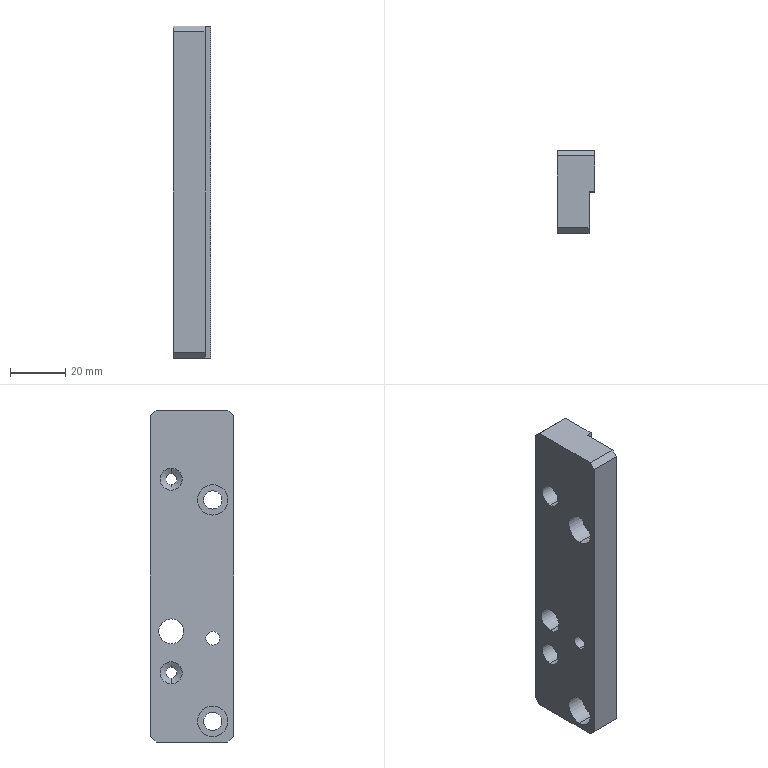Part | SolidWorks | features HoleWzd 5, Chamfer 1, Cut 1, Extrusion 1 | 1 solid | 38 faces | box 13.4 x 30 x 120 mm | volume 40915 mm3 | cylinder 20 | plane 14 | cone 4 | commonest cylinder face diameters 4 x4 6.6 x4 8 x4 11 x4 5 x2 9 x2
STEP:
#1=CARTESIAN_POINT('',(11.4,-7.5,-25.));
#2=VERTEX_POINT('',#1);
#3=CARTESIAN_POINT('',(11.4,-7.5,-20.));
#4=VERTEX_POINT('',#3);
#5=CARTESIAN_POINT('',(11.4,-7.5,-22.5));
#6=DIRECTION('',(-1.,0.,0.));
#7=DIRECTION('',(0.,0.,1.));
#8=AXIS2_PLACEMENT_3D('',#5,#6,#7);
#9=CIRCLE('',#8,2.5);
#10=EDGE_CURVE('',#2,#4,#9,.T.);
#11=ORIENTED_EDGE('',*,*,#10,.F.);
#12=CARTESIAN_POINT('',(0.,-7.5,-25.));
#13=VERTEX_POINT('',#12);
#14=CARTESIAN_POINT('',(0.,-7.5,-25.));
#15=DIRECTION('',(-1.,0.,0.));
#16=VECTOR('',#15,1000.);
#17=LINE('',#14,#16);
#18=EDGE_CURVE('',#2,#13,#17,.T.);
#19=ORIENTED_EDGE('',*,*,#18,.T.);
#20=CARTESIAN_POINT('',(0.,-7.5,-20.));
#21=VERTEX_POINT('',#20);
#22=CARTESIAN_POINT('',(0.,-7.5,-22.5));
#23=DIRECTION('',(-1.,0.,0.));
#24=DIRECTION('',(0.,0.,1.));
#25=AXIS2_PLACEMENT_3D('',#22,#23,#24);
#26=CIRCLE('',#25,2.5);
#27=EDGE_CURVE('',#13,#21,#26,.T.);
#28=ORIENTED_EDGE('',*,*,#27,.T.);
#29=CARTESIAN_POINT('',(0.,-7.5,-20.));
#30=DIRECTION('',(-1.,0.,0.));
#31=VECTOR('',#30,1000.);
#32=LINE('',#29,#31);
#33=EDGE_CURVE('',#4,#21,#32,.T.);
#34=ORIENTED_EDGE('',*,*,#33,.F.);
#35=EDGE_LOOP('',(#11,#19,#28,#34));
#36=FACE_OUTER_BOUND('',#35,.T.);
#37=CARTESIAN_POINT('',(0.,-7.5,-22.5));
#38=DIRECTION('',(-1.,0.,0.));
#39=DIRECTION('',(0.,0.,1.));
#40=AXIS2_PLACEMENT_3D('',#37,#38,#39);
#41=CYLINDRICAL_SURFACE('',#40,2.5);
#42=ADVANCED_FACE('',(#36),#41,.F.);
#43=CARTESIAN_POINT('',(6.8,-7.5,-58.));
#44=VERTEX_POINT('',#43);
#45=CARTESIAN_POINT('',(6.8,-7.5,-47.));
#46=VERTEX_POINT('',#45);
#47=CARTESIAN_POINT('',(6.8,-7.5,-52.5));
#48=DIRECTION('',(-1.,0.,0.));
#49=DIRECTION('',(0.,0.,1.));
#50=AXIS2_PLACEMENT_3D('',#47,#48,#49);
#51=CIRCLE('',#50,5.5);
#52=EDGE_CURVE('',#44,#46,#51,.T.);
#53=ORIENTED_EDGE('',*,*,#52,.F.);
#54=CARTESIAN_POINT('',(0.,-7.5,-58.));
#55=VERTEX_POINT('',#54);
#56=CARTESIAN_POINT('',(0.,-7.5,-58.));
#57=DIRECTION('',(-1.,0.,0.));
#58=VECTOR('',#57,1000.);
#59=LINE('',#56,#58);
#60=EDGE_CURVE('',#44,#55,#59,.T.);
#61=ORIENTED_EDGE('',*,*,#60,.T.);
#62=CARTESIAN_POINT('',(0.,-7.5,-47.));
#63=VERTEX_POINT('',#62);
#64=CARTESIAN_POINT('',(0.,-7.5,-52.5));
#65=DIRECTION('',(-1.,0.,0.));
#66=DIRECTION('',(0.,0.,1.));
#67=AXIS2_PLACEMENT_3D('',#64,#65,#66);
#68=CIRCLE('',#67,5.5);
#69=EDGE_CURVE('',#55,#63,#68,.T.);
#70=ORIENTED_EDGE('',*,*,#69,.T.);
#71=CARTESIAN_POINT('',(0.,-7.5,-47.));
#72=DIRECTION('',(-1.,0.,0.));
#73=VECTOR('',#72,1000.);
#74=LINE('',#71,#73);
#75=EDGE_CURVE('',#46,#63,#74,.T.);
#76=ORIENTED_EDGE('',*,*,#75,.F.);
#77=EDGE_LOOP('',(#53,#61,#70,#76));
#78=FACE_OUTER_BOUND('',#77,.T.);
#79=CARTESIAN_POINT('',(0.,-7.5,-52.5));
#80=DIRECTION('',(-1.,0.,0.));
#81=DIRECTION('',(0.,0.,1.));
#82=AXIS2_PLACEMENT_3D('',#79,#80,#81);
#83=CYLINDRICAL_SURFACE('',#82,5.5);
#84=ADVANCED_FACE('',(#78),#83,.F.);
#85=CARTESIAN_POINT('',(11.4,-7.5,-55.8));
#86=VERTEX_POINT('',#85);
#87=CARTESIAN_POINT('',(11.4,-7.5,-49.2));
#88=VERTEX_POINT('',#87);
#89=CARTESIAN_POINT('',(11.4,-7.5,-52.5));
#90=DIRECTION('',(-1.,0.,0.));
#91=DIRECTION('',(0.,0.,1.));
#92=AXIS2_PLACEMENT_3D('',#89,#90,#91);
#93=CIRCLE('',#92,3.3);
#94=EDGE_CURVE('',#86,#88,#93,.T.);
#95=ORIENTED_EDGE('',*,*,#94,.F.);
#96=CARTESIAN_POINT('',(6.8,-7.5,-55.8));
#97=VERTEX_POINT('',#96);
#98=CARTESIAN_POINT('',(0.,-7.5,-55.8));
#99=DIRECTION('',(-1.,0.,0.));
#100=VECTOR('',#99,1000.);
#101=LINE('',#98,#100);
#102=EDGE_CURVE('',#86,#97,#101,.T.);
#103=ORIENTED_EDGE('',*,*,#102,.T.);
#104=CARTESIAN_POINT('',(6.8,-7.5,-49.2));
#105=VERTEX_POINT('',#104);
#106=CARTESIAN_POINT('',(6.8,-7.5,-52.5));
#107=DIRECTION('',(-1.,0.,0.));
#108=DIRECTION('',(0.,0.,1.));
#109=AXIS2_PLACEMENT_3D('',#106,#107,#108);
#110=CIRCLE('',#109,3.3);
#111=EDGE_CURVE('',#97,#105,#110,.T.);
#112=ORIENTED_EDGE('',*,*,#111,.T.);
#113=CARTESIAN_POINT('',(0.,-7.5,-49.2));
#114=DIRECTION('',(-1.,0.,0.));
#115=VECTOR('',#114,1000.);
#116=LINE('',#113,#115);
#117=EDGE_CURVE('',#88,#105,#116,.T.);
#118=ORIENTED_EDGE('',*,*,#117,.F.);
#119=EDGE_LOOP('',(#95,#103,#112,#118));
#120=FACE_OUTER_BOUND('',#119,.T.);
#121=CARTESIAN_POINT('',(0.,-7.5,-52.5));
#122=DIRECTION('',(-1.,0.,0.));
#123=DIRECTION('',(0.,0.,1.));
#124=AXIS2_PLACEMENT_3D('',#121,#122,#123);
#125=CYLINDRICAL_SURFACE('',#124,3.3);
#126=ADVANCED_FACE('',(#120),#125,.F.);
#127=CARTESIAN_POINT('',(6.8,-7.5,22.));
#128=VERTEX_POINT('',#127);
#129=CARTESIAN_POINT('',(6.8,-7.5,33.));
#130=VERTEX_POINT('',#129);
#131=CARTESIAN_POINT('',(6.8,-7.5,27.5));
#132=DIRECTION('',(-1.,0.,0.));
#133=DIRECTION('',(0.,0.,1.));
#134=AXIS2_PLACEMENT_3D('',#131,#132,#133);
#135=CIRCLE('',#134,5.5);
#136=EDGE_CURVE('',#128,#130,#135,.T.);
#137=ORIENTED_EDGE('',*,*,#136,.F.);
#138=CARTESIAN_POINT('',(0.,-7.5,22.));
#139=VERTEX_POINT('',#138);
#140=CARTESIAN_POINT('',(0.,-7.5,22.));
#141=DIRECTION('',(-1.,0.,0.));
#142=VECTOR('',#141,1000.);
#143=LINE('',#140,#142);
#144=EDGE_CURVE('',#128,#139,#143,.T.);
#145=ORIENTED_EDGE('',*,*,#144,.T.);
#146=CARTESIAN_POINT('',(0.,-7.5,33.));
#147=VERTEX_POINT('',#146);
#148=CARTESIAN_POINT('',(0.,-7.5,27.5));
#149=DIRECTION('',(-1.,0.,0.));
#150=DIRECTION('',(0.,0.,1.));
#151=AXIS2_PLACEMENT_3D('',#148,#149,#150);
#152=CIRCLE('',#151,5.5);
#153=EDGE_CURVE('',#139,#147,#152,.T.);
#154=ORIENTED_EDGE('',*,*,#153,.T.);
#155=CARTESIAN_POINT('',(0.,-7.5,33.));
#156=DIRECTION('',(-1.,0.,0.));
#157=VECTOR('',#156,1000.);
#158=LINE('',#155,#157);
#159=EDGE_CURVE('',#130,#147,#158,.T.);
#160=ORIENTED_EDGE('',*,*,#159,.F.);
#161=EDGE_LOOP('',(#137,#145,#154,#160));
#162=FACE_OUTER_BOUND('',#161,.T.);
#163=CARTESIAN_POINT('',(0.,-7.5,27.5));
#164=DIRECTION('',(-1.,0.,0.));
#165=DIRECTION('',(0.,0.,1.));
#166=AXIS2_PLACEMENT_3D('',#163,#164,#165);
#167=CYLINDRICAL_SURFACE('',#166,5.5);
#168=ADVANCED_FACE('',(#162),#167,.F.);
#169=CARTESIAN_POINT('',(11.4,-7.5,24.2));
#170=VERTEX_POINT('',#169);
#171=CARTESIAN_POINT('',(11.4,-7.5,30.8));
#172=VERTEX_POINT('',#171);
#173=CARTESIAN_POINT('',(11.4,-7.5,27.5));
#174=DIRECTION('',(-1.,0.,0.));
#175=DIRECTION('',(0.,0.,1.));
#176=AXIS2_PLACEMENT_3D('',#173,#174,#175);
#177=CIRCLE('',#176,3.3);
#178=EDGE_CURVE('',#170,#172,#177,.T.);
#179=ORIENTED_EDGE('',*,*,#178,.F.);
#180=CARTESIAN_POINT('',(6.8,-7.5,24.2));
#181=VERTEX_POINT('',#180);
#182=CARTESIAN_POINT('',(0.,-7.5,24.2));
#183=DIRECTION('',(-1.,0.,0.));
#184=VECTOR('',#183,1000.);
#185=LINE('',#182,#184);
#186=EDGE_CURVE('',#170,#181,#185,.T.);
#187=ORIENTED_EDGE('',*,*,#186,.T.);
#188=CARTESIAN_POINT('',(6.8,-7.5,30.8));
#189=VERTEX_POINT('',#188);
#190=CARTESIAN_POINT('',(6.8,-7.5,27.5));
#191=DIRECTION('',(-1.,0.,0.));
#192=DIRECTION('',(0.,0.,1.));
#193=AXIS2_PLACEMENT_3D('',#190,#191,#192);
#194=CIRCLE('',#193,3.3);
#195=EDGE_CURVE('',#181,#189,#194,.T.);
#196=ORIENTED_EDGE('',*,*,#195,.T.);
#197=CARTESIAN_POINT('',(0.,-7.5,30.8));
#198=DIRECTION('',(-1.,0.,0.));
#199=VECTOR('',#198,1000.);
#200=LINE('',#197,#199);
#201=EDGE_CURVE('',#172,#189,#200,.T.);
#202=ORIENTED_EDGE('',*,*,#201,.F.);
#203=EDGE_LOOP('',(#179,#187,#196,#202));
#204=FACE_OUTER_BOUND('',#203,.T.);
#205=CARTESIAN_POINT('',(0.,-7.5,27.5));
#206=DIRECTION('',(-1.,0.,0.));
#207=DIRECTION('',(0.,0.,1.));
#208=AXIS2_PLACEMENT_3D('',#205,#206,#207);
#209=CYLINDRICAL_SURFACE('',#208,3.3);
#210=ADVANCED_FACE('',(#204),#209,.F.);
#211=CARTESIAN_POINT('',(0.,7.5,-15.5));
#212=VERTEX_POINT('',#211);
#213=CARTESIAN_POINT('',(0.,7.5,-24.5));
#214=VERTEX_POINT('',#213);
#215=CARTESIAN_POINT('',(0.,7.5,-20.));
#216=DIRECTION('',(1.,0.,0.));
#217=DIRECTION('',(0.,0.,-1.));
#218=AXIS2_PLACEMENT_3D('',#215,#216,#217);
#219=CIRCLE('',#218,4.5);
#220=EDGE_CURVE('',#212,#214,#219,.T.);
#221=ORIENTED_EDGE('',*,*,#220,.F.);
#222=CARTESIAN_POINT('',(13.4,7.5,-15.5));
#223=VERTEX_POINT('',#222);
#224=CARTESIAN_POINT('',(13.4,7.5,-15.5));
#225=DIRECTION('',(1.,0.,0.));
#226=VECTOR('',#225,1000.);
#227=LINE('',#224,#226);
#228=EDGE_CURVE('',#212,#223,#227,.T.);
#229=ORIENTED_EDGE('',*,*,#228,.T.);
#230=CARTESIAN_POINT('',(13.4,7.5,-24.5));
#231=VERTEX_POINT('',#230);
#232=CARTESIAN_POINT('',(13.4,7.5,-20.));
#233=DIRECTION('',(1.,0.,0.));
#234=DIRECTION('',(0.,0.,-1.));
#235=AXIS2_PLACEMENT_3D('',#232,#233,#234);
#236=CIRCLE('',#235,4.5);
#237=EDGE_CURVE('',#223,#231,#236,.T.);
#238=ORIENTED_EDGE('',*,*,#237,.T.);
#239=CARTESIAN_POINT('',(13.4,7.5,-24.5));
#240=DIRECTION('',(1.,0.,0.));
#241=VECTOR('',#240,1000.);
#242=LINE('',#239,#241);
#243=EDGE_CURVE('',#214,#231,#242,.T.);
#244=ORIENTED_EDGE('',*,*,#243,.F.);
#245=EDGE_LOOP('',(#221,#229,#238,#244));
#246=FACE_OUTER_BOUND('',#245,.T.);
#247=CARTESIAN_POINT('',(13.4,7.5,-20.));
#248=DIRECTION('',(1.,0.,0.));
#249=DIRECTION('',(0.,0.,-1.));
#250=AXIS2_PLACEMENT_3D('',#247,#248,#249);
#251=CYLINDRICAL_SURFACE('',#250,4.5);
#252=ADVANCED_FACE('',(#246),#251,.F.);
#253=CARTESIAN_POINT('',(7.5,7.5,31.));
#254=VERTEX_POINT('',#253);
#255=CARTESIAN_POINT('',(7.5,7.5,39.));
#256=VERTEX_POINT('',#255);
#257=CARTESIAN_POINT('',(7.5,7.5,35.));
#258=DIRECTION('',(-1.,0.,0.));
#259=DIRECTION('',(0.,0.,1.));
#260=AXIS2_PLACEMENT_3D('',#257,#258,#259);
#261=CIRCLE('',#260,4.);
#262=EDGE_CURVE('',#254,#256,#261,.T.);
#263=ORIENTED_EDGE('',*,*,#262,.F.);
#264=CARTESIAN_POINT('',(0.,7.5,31.));
#265=VERTEX_POINT('',#264);
#266=CARTESIAN_POINT('',(0.,7.5,31.));
#267=DIRECTION('',(-1.,0.,0.));
#268=VECTOR('',#267,1000.);
#269=LINE('',#266,#268);
#270=EDGE_CURVE('',#254,#265,#269,.T.);
#271=ORIENTED_EDGE('',*,*,#270,.T.);
#272=CARTESIAN_POINT('',(0.,7.5,39.));
#273=VERTEX_POINT('',#272);
#274=CARTESIAN_POINT('',(0.,7.5,35.));
#275=DIRECTION('',(-1.,0.,0.));
#276=DIRECTION('',(0.,0.,1.));
#277=AXIS2_PLACEMENT_3D('',#274,#275,#276);
#278=CIRCLE('',#277,4.);
#279=EDGE_CURVE('',#265,#273,#278,.T.);
#280=ORIENTED_EDGE('',*,*,#279,.T.);
#281=CARTESIAN_POINT('',(0.,7.5,39.));
#282=DIRECTION('',(-1.,0.,0.));
#283=VECTOR('',#282,1000.);
#284=LINE('',#281,#283);
#285=EDGE_CURVE('',#256,#273,#284,.T.);
#286=ORIENTED_EDGE('',*,*,#285,.F.);
#287=EDGE_LOOP('',(#263,#271,#280,#286));
#288=FACE_OUTER_BOUND('',#287,.T.);
#289=CARTESIAN_POINT('',(0.,7.5,35.));
#290=DIRECTION('',(-1.,0.,0.));
#291=DIRECTION('',(0.,0.,1.));
#292=AXIS2_PLACEMENT_3D('',#289,#290,#291);
#293=CYLINDRICAL_SURFACE('',#292,4.);
#294=ADVANCED_FACE('',(#288),#293,.F.);
#295=CARTESIAN_POINT('',(8.702,7.5,33.));
#296=VERTEX_POINT('',#295);
#297=CARTESIAN_POINT('',(8.702,7.5,37.));
#298=VERTEX_POINT('',#297);
#299=CARTESIAN_POINT('',(8.702,7.5,35.));
#300=DIRECTION('',(-1.,0.,0.));
#301=DIRECTION('',(0.,0.,1.));
#302=AXIS2_PLACEMENT_3D('',#299,#300,#301);
#303=CIRCLE('',#302,2.);
#304=EDGE_CURVE('',#296,#298,#303,.T.);
#305=ORIENTED_EDGE('',*,*,#304,.F.);
#306=CARTESIAN_POINT('',(7.5,7.5,31.));
#307=DIRECTION('',(-0.515,0.,-0.8572));
#308=VECTOR('',#307,1000.);
#309=LINE('',#306,#308);
#310=EDGE_CURVE('',#296,#254,#309,.T.);
#311=ORIENTED_EDGE('',*,*,#310,.T.);
#312=ORIENTED_EDGE('',*,*,#262,.T.);
#313=CARTESIAN_POINT('',(7.5,7.5,39.));
#314=DIRECTION('',(-0.515,0.,0.8572));
#315=VECTOR('',#314,1000.);
#316=LINE('',#313,#315);
#317=EDGE_CURVE('',#298,#256,#316,.T.);
#318=ORIENTED_EDGE('',*,*,#317,.F.);
#319=EDGE_LOOP('',(#305,#311,#312,#318));
#320=FACE_OUTER_BOUND('',#319,.T.);
#321=CARTESIAN_POINT('',(7.5,7.5,35.));
#322=DIRECTION('',(-1.,0.,0.));
#323=DIRECTION('',(0.,0.,1.));
#324=AXIS2_PLACEMENT_3D('',#321,#322,#323);
#325=CONICAL_SURFACE('',#324,4.,1.03);
#326=ADVANCED_FACE('',(#320),#325,.F.);
#327=CARTESIAN_POINT('',(13.4,7.5,33.));
#328=VERTEX_POINT('',#327);
#329=CARTESIAN_POINT('',(13.4,7.5,37.));
#330=VERTEX_POINT('',#329);
#331=CARTESIAN_POINT('',(13.4,7.5,35.));
#332=DIRECTION('',(-1.,0.,0.));
#333=DIRECTION('',(0.,0.,1.));
#334=AXIS2_PLACEMENT_3D('',#331,#332,#333);
#335=CIRCLE('',#334,2.);
#336=EDGE_CURVE('',#328,#330,#335,.T.);
#337=ORIENTED_EDGE('',*,*,#336,.F.);
#338=CARTESIAN_POINT('',(0.,7.5,33.));
#339=DIRECTION('',(-1.,0.,0.));
#340=VECTOR('',#339,1000.);
#341=LINE('',#338,#340);
#342=EDGE_CURVE('',#328,#296,#341,.T.);
#343=ORIENTED_EDGE('',*,*,#342,.T.);
#344=ORIENTED_EDGE('',*,*,#304,.T.);
#345=CARTESIAN_POINT('',(0.,7.5,37.));
#346=DIRECTION('',(-1.,0.,0.));
#347=VECTOR('',#346,1000.);
#348=LINE('',#345,#347);
#349=EDGE_CURVE('',#330,#298,#348,.T.);
#350=ORIENTED_EDGE('',*,*,#349,.F.);
#351=EDGE_LOOP('',(#337,#343,#344,#350));
#352=FACE_OUTER_BOUND('',#351,.T.);
#353=CARTESIAN_POINT('',(0.,7.5,35.));
#354=DIRECTION('',(-1.,0.,0.));
#355=DIRECTION('',(0.,0.,1.));
#356=AXIS2_PLACEMENT_3D('',#353,#354,#355);
#357=CYLINDRICAL_SURFACE('',#356,2.);
#358=ADVANCED_FACE('',(#352),#357,.F.);
#359=CARTESIAN_POINT('',(7.5,7.5,-39.));
#360=VERTEX_POINT('',#359);
#361=CARTESIAN_POINT('',(7.5,7.5,-31.));
#362=VERTEX_POINT('',#361);
#363=CARTESIAN_POINT('',(7.5,7.5,-35.));
#364=DIRECTION('',(-1.,0.,0.));
#365=DIRECTION('',(0.,0.,1.));
#366=AXIS2_PLACEMENT_3D('',#363,#364,#365);
#367=CIRCLE('',#366,4.);
#368=EDGE_CURVE('',#360,#362,#367,.T.);
#369=ORIENTED_EDGE('',*,*,#368,.F.);
#370=CARTESIAN_POINT('',(0.,7.5,-39.));
#371=VERTEX_POINT('',#370);
#372=CARTESIAN_POINT('',(0.,7.5,-39.));
#373=DIRECTION('',(-1.,0.,0.));
#374=VECTOR('',#373,1000.);
#375=LINE('',#372,#374);
#376=EDGE_CURVE('',#360,#371,#375,.T.);
#377=ORIENTED_EDGE('',*,*,#376,.T.);
#378=CARTESIAN_POINT('',(0.,7.5,-31.));
#379=VERTEX_POINT('',#378);
#380=CARTESIAN_POINT('',(0.,7.5,-35.));
#381=DIRECTION('',(-1.,0.,0.));
#382=DIRECTION('',(0.,0.,1.));
#383=AXIS2_PLACEMENT_3D('',#380,#381,#382);
#384=CIRCLE('',#383,4.);
#385=EDGE_CURVE('',#371,#379,#384,.T.);
#386=ORIENTED_EDGE('',*,*,#385,.T.);
#387=CARTESIAN_POINT('',(0.,7.5,-31.));
#388=DIRECTION('',(-1.,0.,0.));
#389=VECTOR('',#388,1000.);
#390=LINE('',#387,#389);
#391=EDGE_CURVE('',#362,#379,#390,.T.);
#392=ORIENTED_EDGE('',*,*,#391,.F.);
#393=EDGE_LOOP('',(#369,#377,#386,#392));
#394=FACE_OUTER_BOUND('',#393,.T.);
#395=CARTESIAN_POINT('',(0.,7.5,-35.));
#396=DIRECTION('',(-1.,0.,0.));
#397=DIRECTION('',(0.,0.,1.));
#398=AXIS2_PLACEMENT_3D('',#395,#396,#397);
#399=CYLINDRICAL_SURFACE('',#398,4.);
#400=ADVANCED_FACE('',(#394),#399,.F.);
#401=CARTESIAN_POINT('',(8.702,7.5,-37.));
#402=VERTEX_POINT('',#401);
#403=CARTESIAN_POINT('',(8.702,7.5,-33.));
#404=VERTEX_POINT('',#403);
#405=CARTESIAN_POINT('',(8.702,7.5,-35.));
#406=DIRECTION('',(-1.,0.,0.));
#407=DIRECTION('',(0.,0.,1.));
#408=AXIS2_PLACEMENT_3D('',#405,#406,#407);
#409=CIRCLE('',#408,2.);
#410=EDGE_CURVE('',#402,#404,#409,.T.);
#411=ORIENTED_EDGE('',*,*,#410,.F.);
#412=CARTESIAN_POINT('',(7.5,7.5,-39.));
#413=DIRECTION('',(-0.515,0.,-0.8572));
#414=VECTOR('',#413,1000.);
#415=LINE('',#412,#414);
#416=EDGE_CURVE('',#402,#360,#415,.T.);
#417=ORIENTED_EDGE('',*,*,#416,.T.);
#418=ORIENTED_EDGE('',*,*,#368,.T.);
#419=CARTESIAN_POINT('',(7.5,7.5,-31.));
#420=DIRECTION('',(-0.515,0.,0.8572));
#421=VECTOR('',#420,1000.);
#422=LINE('',#419,#421);
#423=EDGE_CURVE('',#404,#362,#422,.T.);
#424=ORIENTED_EDGE('',*,*,#423,.F.);
#425=EDGE_LOOP('',(#411,#417,#418,#424));
#426=FACE_OUTER_BOUND('',#425,.T.);
#427=CARTESIAN_POINT('',(7.5,7.5,-35.));
#428=DIRECTION('',(-1.,0.,0.));
#429=DIRECTION('',(0.,0.,1.));
#430=AXIS2_PLACEMENT_3D('',#427,#428,#429);
#431=CONICAL_SURFACE('',#430,4.,1.03);
#432=ADVANCED_FACE('',(#426),#431,.F.);
#433=CARTESIAN_POINT('',(13.4,7.5,-37.));
#434=VERTEX_POINT('',#433);
#435=CARTESIAN_POINT('',(13.4,7.5,-33.));
#436=VERTEX_POINT('',#435);
#437=CARTESIAN_POINT('',(13.4,7.5,-35.));
#438=DIRECTION('',(-1.,0.,0.));
#439=DIRECTION('',(0.,0.,1.));
#440=AXIS2_PLACEMENT_3D('',#437,#438,#439);
#441=CIRCLE('',#440,2.);
#442=EDGE_CURVE('',#434,#436,#441,.T.);
#443=ORIENTED_EDGE('',*,*,#442,.F.);
#444=CARTESIAN_POINT('',(0.,7.5,-37.));
#445=DIRECTION('',(-1.,0.,0.));
#446=VECTOR('',#445,1000.);
#447=LINE('',#444,#446);
#448=EDGE_CURVE('',#434,#402,#447,.T.);
#449=ORIENTED_EDGE('',*,*,#448,.T.);
#450=ORIENTED_EDGE('',*,*,#410,.T.);
#451=CARTESIAN_POINT('',(0.,7.5,-33.));
#452=DIRECTION('',(-1.,0.,0.));
#453=VECTOR('',#452,1000.);
#454=LINE('',#451,#453);
#455=EDGE_CURVE('',#436,#404,#454,.T.);
#456=ORIENTED_EDGE('',*,*,#455,.F.);
#457=EDGE_LOOP('',(#443,#449,#450,#456));
#458=FACE_OUTER_BOUND('',#457,.T.);
#459=CARTESIAN_POINT('',(0.,7.5,-35.));
#460=DIRECTION('',(-1.,0.,0.));
#461=DIRECTION('',(0.,0.,1.));
#462=AXIS2_PLACEMENT_3D('',#459,#460,#461);
#463=CYLINDRICAL_SURFACE('',#462,2.);
#464=ADVANCED_FACE('',(#458),#463,.F.);
#465=CARTESIAN_POINT('',(13.4,7.5,35.));
#466=DIRECTION('',(-1.,0.,0.));
#467=DIRECTION('',(0.,0.,1.));
#468=AXIS2_PLACEMENT_3D('',#465,#466,#467);
#469=CIRCLE('',#468,2.);
#470=EDGE_CURVE('',#330,#328,#469,.T.);
#471=ORIENTED_EDGE('',*,*,#470,.T.);
#472=ORIENTED_EDGE('',*,*,#336,.T.);
#473=EDGE_LOOP('',(#471,#472));
#474=FACE_BOUND('',#473,.T.);
#475=CARTESIAN_POINT('',(13.4,7.5,-35.));
#476=DIRECTION('',(-1.,0.,0.));
#477=DIRECTION('',(0.,0.,1.));
#478=AXIS2_PLACEMENT_3D('',#475,#476,#477);
#479=CIRCLE('',#478,2.);
#480=EDGE_CURVE('',#436,#434,#479,.T.);
#481=ORIENTED_EDGE('',*,*,#480,.T.);
#482=ORIENTED_EDGE('',*,*,#442,.T.);
#483=EDGE_LOOP('',(#481,#482));
#484=FACE_BOUND('',#483,.T.);
#485=CARTESIAN_POINT('',(13.4,0.,-60.));
#486=VERTEX_POINT('',#485);
#487=CARTESIAN_POINT('',(13.4,13.,-60.));
#488=VERTEX_POINT('',#487);
#489=CARTESIAN_POINT('',(13.4,-15.,-60.));
#490=DIRECTION('',(0.,1.,0.));
#491=VECTOR('',#490,1000.);
#492=LINE('',#489,#491);
#493=EDGE_CURVE('',#486,#488,#492,.T.);
#494=ORIENTED_EDGE('',*,*,#493,.T.);
#495=CARTESIAN_POINT('',(13.4,15.,-58.));
#496=VERTEX_POINT('',#495);
#497=CARTESIAN_POINT('',(13.4,15.,-58.));
#498=DIRECTION('',(0.,0.7071,0.7071));
#499=VECTOR('',#498,1000.);
#500=LINE('',#497,#499);
#501=EDGE_CURVE('',#488,#496,#500,.T.);
#502=ORIENTED_EDGE('',*,*,#501,.T.);
#503=CARTESIAN_POINT('',(13.4,15.,58.));
#504=VERTEX_POINT('',#503);
#505=CARTESIAN_POINT('',(13.4,15.,60.));
#506=DIRECTION('',(0.,0.,1.));
#507=VECTOR('',#506,1000.);
#508=LINE('',#505,#507);
#509=EDGE_CURVE('',#496,#504,#508,.T.);
#510=ORIENTED_EDGE('',*,*,#509,.T.);
#511=CARTESIAN_POINT('',(13.4,13.,60.));
#512=VERTEX_POINT('',#511);
#513=CARTESIAN_POINT('',(13.4,13.,60.));
#514=DIRECTION('',(0.,-0.7071,0.7071));
#515=VECTOR('',#514,1000.);
#516=LINE('',#513,#515);
#517=EDGE_CURVE('',#504,#512,#516,.T.);
#518=ORIENTED_EDGE('',*,*,#517,.T.);
#519=CARTESIAN_POINT('',(13.4,0.,60.));
#520=VERTEX_POINT('',#519);
#521=CARTESIAN_POINT('',(13.4,-15.,60.));
#522=DIRECTION('',(0.,-1.,0.));
#523=VECTOR('',#522,1000.);
#524=LINE('',#521,#523);
#525=EDGE_CURVE('',#512,#520,#524,.T.);
#526=ORIENTED_EDGE('',*,*,#525,.T.);
#527=CARTESIAN_POINT('',(13.4,0.,60.));
#528=DIRECTION('',(0.,0.,1.));
#529=VECTOR('',#528,1000.);
#530=LINE('',#527,#529);
#531=EDGE_CURVE('',#486,#520,#530,.T.);
#532=ORIENTED_EDGE('',*,*,#531,.F.);
#533=EDGE_LOOP('',(#494,#502,#510,#518,#526,#532));
#534=FACE_OUTER_BOUND('',#533,.T.);
#535=CARTESIAN_POINT('',(13.4,7.5,-20.));
#536=DIRECTION('',(1.,0.,0.));
#537=DIRECTION('',(0.,0.,-1.));
#538=AXIS2_PLACEMENT_3D('',#535,#536,#537);
#539=CIRCLE('',#538,4.5);
#540=EDGE_CURVE('',#231,#223,#539,.T.);
#541=ORIENTED_EDGE('',*,*,#540,.F.);
#542=ORIENTED_EDGE('',*,*,#237,.F.);
#543=EDGE_LOOP('',(#541,#542));
#544=FACE_BOUND('',#543,.T.);
#545=CARTESIAN_POINT('',(13.4,0.,0.));
#546=DIRECTION('',(-1.,0.,0.));
#547=DIRECTION('',(0.,0.,1.));
#548=AXIS2_PLACEMENT_3D('',#545,#546,#547);
#549=PLANE('',#548);
#550=ADVANCED_FACE('',(#474,#484,#534,#544),#549,.F.);
#551=CARTESIAN_POINT('',(11.4,-13.,-60.));
#552=VERTEX_POINT('',#551);
#553=CARTESIAN_POINT('',(11.4,0.,-60.));
#554=VERTEX_POINT('',#553);
#555=CARTESIAN_POINT('',(11.4,-15.,-60.));
#556=DIRECTION('',(0.,1.,0.));
#557=VECTOR('',#556,1000.);
#558=LINE('',#555,#557);
#559=EDGE_CURVE('',#552,#554,#558,.T.);
#560=ORIENTED_EDGE('',*,*,#559,.F.);
#561=CARTESIAN_POINT('',(0.,-13.,-60.));
#562=VERTEX_POINT('',#561);
#563=CARTESIAN_POINT('',(13.4,-13.,-60.));
#564=DIRECTION('',(-1.,0.,0.));
#565=VECTOR('',#564,1000.);
#566=LINE('',#563,#565);
#567=EDGE_CURVE('',#552,#562,#566,.T.);
#568=ORIENTED_EDGE('',*,*,#567,.T.);
#569=CARTESIAN_POINT('',(0.,13.,-60.));
#570=VERTEX_POINT('',#569);
#571=CARTESIAN_POINT('',(0.,-15.,-60.));
#572=DIRECTION('',(0.,1.,0.));
#573=VECTOR('',#572,1000.);
#574=LINE('',#571,#573);
#575=EDGE_CURVE('',#562,#570,#574,.T.);
#576=ORIENTED_EDGE('',*,*,#575,.T.);
#577=CARTESIAN_POINT('',(13.4,13.,-60.));
#578=DIRECTION('',(1.,0.,0.));
#579=VECTOR('',#578,1000.);
#580=LINE('',#577,#579);
#581=EDGE_CURVE('',#570,#488,#580,.T.);
#582=ORIENTED_EDGE('',*,*,#581,.T.);
#583=ORIENTED_EDGE('',*,*,#493,.F.);
#584=CARTESIAN_POINT('',(11.4,0.,-60.));
#585=DIRECTION('',(1.,0.,0.));
#586=VECTOR('',#585,1000.);
#587=LINE('',#584,#586);
#588=EDGE_CURVE('',#554,#486,#587,.T.);
#589=ORIENTED_EDGE('',*,*,#588,.F.);
#590=EDGE_LOOP('',(#560,#568,#576,#582,#583,#589));
#591=FACE_OUTER_BOUND('',#590,.T.);
#592=CARTESIAN_POINT('',(13.4,-15.,-60.));
#593=DIRECTION('',(0.,0.,1.));
#594=DIRECTION('',(1.,0.,0.));
#595=AXIS2_PLACEMENT_3D('',#592,#593,#594);
#596=PLANE('',#595);
#597=ADVANCED_FACE('',(#591),#596,.F.);
#598=ORIENTED_EDGE('',*,*,#509,.F.);
#599=CARTESIAN_POINT('',(0.,15.,-58.));
#600=VERTEX_POINT('',#599);
#601=CARTESIAN_POINT('',(13.4,15.,-58.));
#602=DIRECTION('',(-1.,0.,0.));
#603=VECTOR('',#602,1000.);
#604=LINE('',#601,#603);
#605=EDGE_CURVE('',#496,#600,#604,.T.);
#606=ORIENTED_EDGE('',*,*,#605,.T.);
#607=CARTESIAN_POINT('',(0.,15.,58.));
#608=VERTEX_POINT('',#607);
#609=CARTESIAN_POINT('',(0.,15.,60.));
#610=DIRECTION('',(0.,0.,1.));
#611=VECTOR('',#610,1000.);
#612=LINE('',#609,#611);
#613=EDGE_CURVE('',#600,#608,#612,.T.);
#614=ORIENTED_EDGE('',*,*,#613,.T.);
#615=CARTESIAN_POINT('',(13.4,15.,58.));
#616=DIRECTION('',(1.,0.,0.));
#617=VECTOR('',#616,1000.);
#618=LINE('',#615,#617);
#619=EDGE_CURVE('',#608,#504,#618,.T.);
#620=ORIENTED_EDGE('',*,*,#619,.T.);
#621=EDGE_LOOP('',(#598,#606,#614,#620));
#622=FACE_OUTER_BOUND('',#621,.T.);
#623=CARTESIAN_POINT('',(13.4,15.,60.));
#624=DIRECTION('',(0.,-1.,0.));
#625=DIRECTION('',(0.,0.,-1.));
#626=AXIS2_PLACEMENT_3D('',#623,#624,#625);
#627=PLANE('',#626);
#628=ADVANCED_FACE('',(#622),#627,.F.);
#629=CARTESIAN_POINT('',(0.,13.,60.));
#630=VERTEX_POINT('',#629);
#631=CARTESIAN_POINT('',(0.,-13.,60.));
#632=VERTEX_POINT('',#631);
#633=CARTESIAN_POINT('',(0.,-15.,60.));
#634=DIRECTION('',(0.,-1.,0.));
#635=VECTOR('',#634,1000.);
#636=LINE('',#633,#635);
#637=EDGE_CURVE('',#630,#632,#636,.T.);
#638=ORIENTED_EDGE('',*,*,#637,.T.);
#639=CARTESIAN_POINT('',(11.4,-13.,60.));
#640=VERTEX_POINT('',#639);
#641=CARTESIAN_POINT('',(13.4,-13.,60.));
#642=DIRECTION('',(1.,0.,0.));
#643=VECTOR('',#642,1000.);
#644=LINE('',#641,#643);
#645=EDGE_CURVE('',#632,#640,#644,.T.);
#646=ORIENTED_EDGE('',*,*,#645,.T.);
#647=CARTESIAN_POINT('',(11.4,0.,60.));
#648=VERTEX_POINT('',#647);
#649=CARTESIAN_POINT('',(11.4,-15.,60.));
#650=DIRECTION('',(0.,-1.,0.));
#651=VECTOR('',#650,1000.);
#652=LINE('',#649,#651);
#653=EDGE_CURVE('',#648,#640,#652,.T.);
#654=ORIENTED_EDGE('',*,*,#653,.F.);
#655=CARTESIAN_POINT('',(11.4,0.,60.));
#656=DIRECTION('',(1.,0.,0.));
#657=VECTOR('',#656,1000.);
#658=LINE('',#655,#657);
#659=EDGE_CURVE('',#648,#520,#658,.T.);
#660=ORIENTED_EDGE('',*,*,#659,.T.);
#661=ORIENTED_EDGE('',*,*,#525,.F.);
#662=CARTESIAN_POINT('',(13.4,13.,60.));
#663=DIRECTION('',(-1.,0.,0.));
#664=VECTOR('',#663,1000.);
#665=LINE('',#662,#664);
#666=EDGE_CURVE('',#512,#630,#665,.T.);
#667=ORIENTED_EDGE('',*,*,#666,.T.);
#668=EDGE_LOOP('',(#638,#646,#654,#660,#661,#667));
#669=FACE_OUTER_BOUND('',#668,.T.);
#670=CARTESIAN_POINT('',(13.4,-15.,60.));
#671=DIRECTION('',(0.,0.,-1.));
#672=DIRECTION('',(-1.,0.,0.));
#673=AXIS2_PLACEMENT_3D('',#670,#671,#672);
#674=PLANE('',#673);
#675=ADVANCED_FACE('',(#669),#674,.F.);
#676=CARTESIAN_POINT('',(0.,-15.,58.));
#677=VERTEX_POINT('',#676);
#678=CARTESIAN_POINT('',(0.,-15.,-58.));
#679=VERTEX_POINT('',#678);
#680=CARTESIAN_POINT('',(0.,-15.,60.));
#681=DIRECTION('',(0.,0.,-1.));
#682=VECTOR('',#681,1000.);
#683=LINE('',#680,#682);
#684=EDGE_CURVE('',#677,#679,#683,.T.);
#685=ORIENTED_EDGE('',*,*,#684,.T.);
#686=CARTESIAN_POINT('',(11.4,-15.,-58.));
#687=VERTEX_POINT('',#686);
#688=CARTESIAN_POINT('',(13.4,-15.,-58.));
#689=DIRECTION('',(1.,0.,0.));
#690=VECTOR('',#689,1000.);
#691=LINE('',#688,#690);
#692=EDGE_CURVE('',#679,#687,#691,.T.);
#693=ORIENTED_EDGE('',*,*,#692,.T.);
#694=CARTESIAN_POINT('',(11.4,-15.,58.));
#695=VERTEX_POINT('',#694);
#696=CARTESIAN_POINT('',(11.4,-15.,60.));
#697=DIRECTION('',(0.,0.,-1.));
#698=VECTOR('',#697,1000.);
#699=LINE('',#696,#698);
#700=EDGE_CURVE('',#695,#687,#699,.T.);
#701=ORIENTED_EDGE('',*,*,#700,.F.);
#702=CARTESIAN_POINT('',(13.4,-15.,58.));
#703=DIRECTION('',(-1.,0.,0.));
#704=VECTOR('',#703,1000.);
#705=LINE('',#702,#704);
#706=EDGE_CURVE('',#695,#677,#705,.T.);
#707=ORIENTED_EDGE('',*,*,#706,.T.);
#708=EDGE_LOOP('',(#685,#693,#701,#707));
#709=FACE_OUTER_BOUND('',#708,.T.);
#710=CARTESIAN_POINT('',(13.4,-15.,60.));
#711=DIRECTION('',(0.,1.,0.));
#712=DIRECTION('',(0.,0.,1.));
#713=AXIS2_PLACEMENT_3D('',#710,#711,#712);
#714=PLANE('',#713);
#715=ADVANCED_FACE('',(#709),#714,.F.);
#716=CARTESIAN_POINT('',(0.,-7.5,-22.5));
#717=DIRECTION('',(-1.,0.,0.));
#718=DIRECTION('',(0.,0.,1.));
#719=AXIS2_PLACEMENT_3D('',#716,#717,#718);
#720=CIRCLE('',#719,2.5);
#721=EDGE_CURVE('',#21,#13,#720,.T.);
#722=ORIENTED_EDGE('',*,*,#721,.F.);
#723=ORIENTED_EDGE('',*,*,#27,.F.);
#724=EDGE_LOOP('',(#722,#723));
#725=FACE_BOUND('',#724,.T.);
#726=CARTESIAN_POINT('',(0.,-7.5,-52.5));
#727=DIRECTION('',(-1.,0.,0.));
#728=DIRECTION('',(0.,0.,1.));
#729=AXIS2_PLACEMENT_3D('',#726,#727,#728);
#730=CIRCLE('',#729,5.5);
#731=EDGE_CURVE('',#63,#55,#730,.T.);
#732=ORIENTED_EDGE('',*,*,#731,.F.);
#733=ORIENTED_EDGE('',*,*,#69,.F.);
#734=EDGE_LOOP('',(#732,#733));
#735=FACE_BOUND('',#734,.T.);
#736=CARTESIAN_POINT('',(0.,-7.5,27.5));
#737=DIRECTION('',(-1.,0.,0.));
#738=DIRECTION('',(0.,0.,1.));
#739=AXIS2_PLACEMENT_3D('',#736,#737,#738);
#740=CIRCLE('',#739,5.5);
#741=EDGE_CURVE('',#147,#139,#740,.T.);
#742=ORIENTED_EDGE('',*,*,#741,.F.);
#743=ORIENTED_EDGE('',*,*,#153,.F.);
#744=EDGE_LOOP('',(#742,#743));
#745=FACE_BOUND('',#744,.T.);
#746=CARTESIAN_POINT('',(0.,7.5,-20.));
#747=DIRECTION('',(1.,0.,0.));
#748=DIRECTION('',(0.,0.,-1.));
#749=AXIS2_PLACEMENT_3D('',#746,#747,#748);
#750=CIRCLE('',#749,4.5);
#751=EDGE_CURVE('',#214,#212,#750,.T.);
#752=ORIENTED_EDGE('',*,*,#751,.T.);
#753=ORIENTED_EDGE('',*,*,#220,.T.);
#754=EDGE_LOOP('',(#752,#753));
#755=FACE_BOUND('',#754,.T.);
#756=CARTESIAN_POINT('',(0.,7.5,35.));
#757=DIRECTION('',(-1.,0.,0.));
#758=DIRECTION('',(0.,0.,1.));
#759=AXIS2_PLACEMENT_3D('',#756,#757,#758);
#760=CIRCLE('',#759,4.);
#761=EDGE_CURVE('',#273,#265,#760,.T.);
#762=ORIENTED_EDGE('',*,*,#761,.F.);
#763=ORIENTED_EDGE('',*,*,#279,.F.);
#764=EDGE_LOOP('',(#762,#763));
#765=FACE_BOUND('',#764,.T.);
#766=CARTESIAN_POINT('',(0.,7.5,-35.));
#767=DIRECTION('',(-1.,0.,0.));
#768=DIRECTION('',(0.,0.,1.));
#769=AXIS2_PLACEMENT_3D('',#766,#767,#768);
#770=CIRCLE('',#769,4.);
#771=EDGE_CURVE('',#379,#371,#770,.T.);
#772=ORIENTED_EDGE('',*,*,#771,.F.);
#773=ORIENTED_EDGE('',*,*,#385,.F.);
#774=EDGE_LOOP('',(#772,#773));
#775=FACE_BOUND('',#774,.T.);
#776=ORIENTED_EDGE('',*,*,#575,.F.);
#777=CARTESIAN_POINT('',(0.,-36.5,-36.5));
#778=DIRECTION('',(0.,-0.7071,0.7071));
#779=VECTOR('',#778,1000.);
#780=LINE('',#777,#779);
#781=EDGE_CURVE('',#562,#679,#780,.T.);
#782=ORIENTED_EDGE('',*,*,#781,.T.);
#783=ORIENTED_EDGE('',*,*,#684,.F.);
#784=CARTESIAN_POINT('',(0.,-36.5,36.5));
#785=DIRECTION('',(0.,0.7071,0.7071));
#786=VECTOR('',#785,1000.);
#787=LINE('',#784,#786);
#788=EDGE_CURVE('',#677,#632,#787,.T.);
#789=ORIENTED_EDGE('',*,*,#788,.T.);
#790=ORIENTED_EDGE('',*,*,#637,.F.);
#791=CARTESIAN_POINT('',(0.,36.5,36.5));
#792=DIRECTION('',(0.,0.7071,-0.7071));
#793=VECTOR('',#792,1000.);
#794=LINE('',#791,#793);
#795=EDGE_CURVE('',#630,#608,#794,.T.);
#796=ORIENTED_EDGE('',*,*,#795,.T.);
#797=ORIENTED_EDGE('',*,*,#613,.F.);
#798=CARTESIAN_POINT('',(0.,36.5,-36.5));
#799=DIRECTION('',(0.,-0.7071,-0.7071));
#800=VECTOR('',#799,1000.);
#801=LINE('',#798,#800);
#802=EDGE_CURVE('',#600,#570,#801,.T.);
#803=ORIENTED_EDGE('',*,*,#802,.T.);
#804=EDGE_LOOP('',(#776,#782,#783,#789,#790,#796,#797,#803));
#805=FACE_OUTER_BOUND('',#804,.T.);
#806=CARTESIAN_POINT('',(0.,0.,0.));
#807=DIRECTION('',(-1.,0.,0.));
#808=DIRECTION('',(0.,0.,1.));
#809=AXIS2_PLACEMENT_3D('',#806,#807,#808);
#810=PLANE('',#809);
#811=ADVANCED_FACE('',(#725,#735,#745,#755,#765,#775,#805),#810,.T.);
#812=ORIENTED_EDGE('',*,*,#531,.T.);
#813=ORIENTED_EDGE('',*,*,#659,.F.);
#814=CARTESIAN_POINT('',(11.4,0.,60.));
#815=DIRECTION('',(0.,0.,1.));
#816=VECTOR('',#815,1000.);
#817=LINE('',#814,#816);
#818=EDGE_CURVE('',#554,#648,#817,.T.);
#819=ORIENTED_EDGE('',*,*,#818,.F.);
#820=ORIENTED_EDGE('',*,*,#588,.T.);
#821=EDGE_LOOP('',(#812,#813,#819,#820));
#822=FACE_OUTER_BOUND('',#821,.T.);
#823=CARTESIAN_POINT('',(11.4,0.,60.));
#824=DIRECTION('',(0.,1.,0.));
#825=DIRECTION('',(0.,0.,1.));
#826=AXIS2_PLACEMENT_3D('',#823,#824,#825);
#827=PLANE('',#826);
#828=ADVANCED_FACE('',(#822),#827,.F.);
#829=CARTESIAN_POINT('',(11.4,-7.5,-22.5));
#830=DIRECTION('',(-1.,0.,0.));
#831=DIRECTION('',(0.,0.,1.));
#832=AXIS2_PLACEMENT_3D('',#829,#830,#831);
#833=CIRCLE('',#832,2.5);
#834=EDGE_CURVE('',#4,#2,#833,.T.);
#835=ORIENTED_EDGE('',*,*,#834,.T.);
#836=ORIENTED_EDGE('',*,*,#10,.T.);
#837=EDGE_LOOP('',(#835,#836));
#838=FACE_BOUND('',#837,.T.);
#839=CARTESIAN_POINT('',(11.4,-7.5,-52.5));
#840=DIRECTION('',(-1.,0.,0.));
#841=DIRECTION('',(0.,0.,1.));
#842=AXIS2_PLACEMENT_3D('',#839,#840,#841);
#843=CIRCLE('',#842,3.3);
#844=EDGE_CURVE('',#88,#86,#843,.T.);
#845=ORIENTED_EDGE('',*,*,#844,.T.);
#846=ORIENTED_EDGE('',*,*,#94,.T.);
#847=EDGE_LOOP('',(#845,#846));
#848=FACE_BOUND('',#847,.T.);
#849=CARTESIAN_POINT('',(11.4,-7.5,27.5));
#850=DIRECTION('',(-1.,0.,0.));
#851=DIRECTION('',(0.,0.,1.));
#852=AXIS2_PLACEMENT_3D('',#849,#850,#851);
#853=CIRCLE('',#852,3.3);
#854=EDGE_CURVE('',#172,#170,#853,.T.);
#855=ORIENTED_EDGE('',*,*,#854,.T.);
#856=ORIENTED_EDGE('',*,*,#178,.T.);
#857=EDGE_LOOP('',(#855,#856));
#858=FACE_BOUND('',#857,.T.);
#859=ORIENTED_EDGE('',*,*,#700,.T.);
#860=CARTESIAN_POINT('',(11.4,-13.,-60.));
#861=DIRECTION('',(0.,0.7071,-0.7071));
#862=VECTOR('',#861,1000.);
#863=LINE('',#860,#862);
#864=EDGE_CURVE('',#687,#552,#863,.T.);
#865=ORIENTED_EDGE('',*,*,#864,.T.);
#866=ORIENTED_EDGE('',*,*,#559,.T.);
#867=ORIENTED_EDGE('',*,*,#818,.T.);
#868=ORIENTED_EDGE('',*,*,#653,.T.);
#869=CARTESIAN_POINT('',(11.4,-15.,58.));
#870=DIRECTION('',(0.,-0.7071,-0.7071));
#871=VECTOR('',#870,1000.);
#872=LINE('',#869,#871);
#873=EDGE_CURVE('',#640,#695,#872,.T.);
#874=ORIENTED_EDGE('',*,*,#873,.T.);
#875=EDGE_LOOP('',(#859,#865,#866,#867,#868,#874));
#876=FACE_OUTER_BOUND('',#875,.T.);
#877=CARTESIAN_POINT('',(11.4,0.,0.));
#878=DIRECTION('',(-1.,0.,0.));
#879=DIRECTION('',(0.,0.,1.));
#880=AXIS2_PLACEMENT_3D('',#877,#878,#879);
#881=PLANE('',#880);
#882=ADVANCED_FACE('',(#838,#848,#858,#876),#881,.F.);
#883=ORIENTED_EDGE('',*,*,#448,.F.);
#884=ORIENTED_EDGE('',*,*,#480,.F.);
#885=ORIENTED_EDGE('',*,*,#455,.T.);
#886=CARTESIAN_POINT('',(8.702,7.5,-35.));
#887=DIRECTION('',(-1.,0.,0.));
#888=DIRECTION('',(0.,0.,1.));
#889=AXIS2_PLACEMENT_3D('',#886,#887,#888);
#890=CIRCLE('',#889,2.);
#891=EDGE_CURVE('',#404,#402,#890,.T.);
#892=ORIENTED_EDGE('',*,*,#891,.T.);
#893=EDGE_LOOP('',(#883,#884,#885,#892));
#894=FACE_OUTER_BOUND('',#893,.T.);
#895=CARTESIAN_POINT('',(0.,7.5,-35.));
#896=DIRECTION('',(-1.,0.,0.));
#897=DIRECTION('',(0.,0.,1.));
#898=AXIS2_PLACEMENT_3D('',#895,#896,#897);
#899=CYLINDRICAL_SURFACE('',#898,2.);
#900=ADVANCED_FACE('',(#894),#899,.F.);
#901=ORIENTED_EDGE('',*,*,#416,.F.);
#902=ORIENTED_EDGE('',*,*,#891,.F.);
#903=ORIENTED_EDGE('',*,*,#423,.T.);
#904=CARTESIAN_POINT('',(7.5,7.5,-35.));
#905=DIRECTION('',(-1.,0.,0.));
#906=DIRECTION('',(0.,0.,1.));
#907=AXIS2_PLACEMENT_3D('',#904,#905,#906);
#908=CIRCLE('',#907,4.);
#909=EDGE_CURVE('',#362,#360,#908,.T.);
#910=ORIENTED_EDGE('',*,*,#909,.T.);
#911=EDGE_LOOP('',(#901,#902,#903,#910));
#912=FACE_OUTER_BOUND('',#911,.T.);
#913=CARTESIAN_POINT('',(7.5,7.5,-35.));
#914=DIRECTION('',(-1.,0.,0.));
#915=DIRECTION('',(0.,0.,1.));
#916=AXIS2_PLACEMENT_3D('',#913,#914,#915);
#917=CONICAL_SURFACE('',#916,4.,1.03);
#918=ADVANCED_FACE('',(#912),#917,.F.);
#919=ORIENTED_EDGE('',*,*,#376,.F.);
#920=ORIENTED_EDGE('',*,*,#909,.F.);
#921=ORIENTED_EDGE('',*,*,#391,.T.);
#922=ORIENTED_EDGE('',*,*,#771,.T.);
#923=EDGE_LOOP('',(#919,#920,#921,#922));
#924=FACE_OUTER_BOUND('',#923,.T.);
#925=CARTESIAN_POINT('',(0.,7.5,-35.));
#926=DIRECTION('',(-1.,0.,0.));
#927=DIRECTION('',(0.,0.,1.));
#928=AXIS2_PLACEMENT_3D('',#925,#926,#927);
#929=CYLINDRICAL_SURFACE('',#928,4.);
#930=ADVANCED_FACE('',(#924),#929,.F.);
#931=ORIENTED_EDGE('',*,*,#342,.F.);
#932=ORIENTED_EDGE('',*,*,#470,.F.);
#933=ORIENTED_EDGE('',*,*,#349,.T.);
#934=CARTESIAN_POINT('',(8.702,7.5,35.));
#935=DIRECTION('',(-1.,0.,0.));
#936=DIRECTION('',(0.,0.,1.));
#937=AXIS2_PLACEMENT_3D('',#934,#935,#936);
#938=CIRCLE('',#937,2.);
#939=EDGE_CURVE('',#298,#296,#938,.T.);
#940=ORIENTED_EDGE('',*,*,#939,.T.);
#941=EDGE_LOOP('',(#931,#932,#933,#940));
#942=FACE_OUTER_BOUND('',#941,.T.);
#943=CARTESIAN_POINT('',(0.,7.5,35.));
#944=DIRECTION('',(-1.,0.,0.));
#945=DIRECTION('',(0.,0.,1.));
#946=AXIS2_PLACEMENT_3D('',#943,#944,#945);
#947=CYLINDRICAL_SURFACE('',#946,2.);
#948=ADVANCED_FACE('',(#942),#947,.F.);
#949=ORIENTED_EDGE('',*,*,#310,.F.);
#950=ORIENTED_EDGE('',*,*,#939,.F.);
#951=ORIENTED_EDGE('',*,*,#317,.T.);
#952=CARTESIAN_POINT('',(7.5,7.5,35.));
#953=DIRECTION('',(-1.,0.,0.));
#954=DIRECTION('',(0.,0.,1.));
#955=AXIS2_PLACEMENT_3D('',#952,#953,#954);
#956=CIRCLE('',#955,4.);
#957=EDGE_CURVE('',#256,#254,#956,.T.);
#958=ORIENTED_EDGE('',*,*,#957,.T.);
#959=EDGE_LOOP('',(#949,#950,#951,#958));
#960=FACE_OUTER_BOUND('',#959,.T.);
#961=CARTESIAN_POINT('',(7.5,7.5,35.));
#962=DIRECTION('',(-1.,0.,0.));
#963=DIRECTION('',(0.,0.,1.));
#964=AXIS2_PLACEMENT_3D('',#961,#962,#963);
#965=CONICAL_SURFACE('',#964,4.,1.03);
#966=ADVANCED_FACE('',(#960),#965,.F.);
#967=ORIENTED_EDGE('',*,*,#270,.F.);
#968=ORIENTED_EDGE('',*,*,#957,.F.);
#969=ORIENTED_EDGE('',*,*,#285,.T.);
#970=ORIENTED_EDGE('',*,*,#761,.T.);
#971=EDGE_LOOP('',(#967,#968,#969,#970));
#972=FACE_OUTER_BOUND('',#971,.T.);
#973=CARTESIAN_POINT('',(0.,7.5,35.));
#974=DIRECTION('',(-1.,0.,0.));
#975=DIRECTION('',(0.,0.,1.));
#976=AXIS2_PLACEMENT_3D('',#973,#974,#975);
#977=CYLINDRICAL_SURFACE('',#976,4.);
#978=ADVANCED_FACE('',(#972),#977,.F.);
#979=ORIENTED_EDGE('',*,*,#228,.F.);
#980=ORIENTED_EDGE('',*,*,#751,.F.);
#981=ORIENTED_EDGE('',*,*,#243,.T.);
#982=ORIENTED_EDGE('',*,*,#540,.T.);
#983=EDGE_LOOP('',(#979,#980,#981,#982));
#984=FACE_OUTER_BOUND('',#983,.T.);
#985=CARTESIAN_POINT('',(13.4,7.5,-20.));
#986=DIRECTION('',(1.,0.,0.));
#987=DIRECTION('',(0.,0.,-1.));
#988=AXIS2_PLACEMENT_3D('',#985,#986,#987);
#989=CYLINDRICAL_SURFACE('',#988,4.5);
#990=ADVANCED_FACE('',(#984),#989,.F.);
#991=ORIENTED_EDGE('',*,*,#864,.F.);
#992=ORIENTED_EDGE('',*,*,#692,.F.);
#993=ORIENTED_EDGE('',*,*,#781,.F.);
#994=ORIENTED_EDGE('',*,*,#567,.F.);
#995=EDGE_LOOP('',(#991,#992,#993,#994));
#996=FACE_OUTER_BOUND('',#995,.T.);
#997=CARTESIAN_POINT('',(13.4,-13.,-60.));
#998=DIRECTION('',(0.,0.7071,0.7071));
#999=DIRECTION('',(-1.,0.,0.));
#1000=AXIS2_PLACEMENT_3D('',#997,#998,#999);
#1001=PLANE('',#1000);
#1002=ADVANCED_FACE('',(#996),#1001,.F.);
#1003=ORIENTED_EDGE('',*,*,#501,.F.);
#1004=ORIENTED_EDGE('',*,*,#581,.F.);
#1005=ORIENTED_EDGE('',*,*,#802,.F.);
#1006=ORIENTED_EDGE('',*,*,#605,.F.);
#1007=EDGE_LOOP('',(#1003,#1004,#1005,#1006));
#1008=FACE_OUTER_BOUND('',#1007,.T.);
#1009=CARTESIAN_POINT('',(13.4,15.,-58.));
#1010=DIRECTION('',(0.,-0.7071,0.7071));
#1011=DIRECTION('',(-1.,0.,0.));
#1012=AXIS2_PLACEMENT_3D('',#1009,#1010,#1011);
#1013=PLANE('',#1012);
#1014=ADVANCED_FACE('',(#1008),#1013,.F.);
#1015=ORIENTED_EDGE('',*,*,#873,.F.);
#1016=ORIENTED_EDGE('',*,*,#645,.F.);
#1017=ORIENTED_EDGE('',*,*,#788,.F.);
#1018=ORIENTED_EDGE('',*,*,#706,.F.);
#1019=EDGE_LOOP('',(#1015,#1016,#1017,#1018));
#1020=FACE_OUTER_BOUND('',#1019,.T.);
#1021=CARTESIAN_POINT('',(13.4,-15.,58.));
#1022=DIRECTION('',(0.,0.7071,-0.7071));
#1023=DIRECTION('',(-1.,0.,0.));
#1024=AXIS2_PLACEMENT_3D('',#1021,#1022,#1023);
#1025=PLANE('',#1024);
#1026=ADVANCED_FACE('',(#1020),#1025,.F.);
#1027=ORIENTED_EDGE('',*,*,#517,.F.);
#1028=ORIENTED_EDGE('',*,*,#619,.F.);
#1029=ORIENTED_EDGE('',*,*,#795,.F.);
#1030=ORIENTED_EDGE('',*,*,#666,.F.);
#1031=EDGE_LOOP('',(#1027,#1028,#1029,#1030));
#1032=FACE_OUTER_BOUND('',#1031,.T.);
#1033=CARTESIAN_POINT('',(13.4,13.,60.));
#1034=DIRECTION('',(0.,-0.7071,-0.7071));
#1035=DIRECTION('',(-1.,0.,0.));
#1036=AXIS2_PLACEMENT_3D('',#1033,#1034,#1035);
#1037=PLANE('',#1036);
#1038=ADVANCED_FACE('',(#1032),#1037,.F.);
#1039=ORIENTED_EDGE('',*,*,#186,.F.);
#1040=ORIENTED_EDGE('',*,*,#854,.F.);
#1041=ORIENTED_EDGE('',*,*,#201,.T.);
#1042=CARTESIAN_POINT('',(6.8,-7.5,27.5));
#1043=DIRECTION('',(-1.,0.,0.));
#1044=DIRECTION('',(0.,0.,1.));
#1045=AXIS2_PLACEMENT_3D('',#1042,#1043,#1044);
#1046=CIRCLE('',#1045,3.3);
#1047=EDGE_CURVE('',#189,#181,#1046,.T.);
#1048=ORIENTED_EDGE('',*,*,#1047,.T.);
#1049=EDGE_LOOP('',(#1039,#1040,#1041,#1048));
#1050=FACE_OUTER_BOUND('',#1049,.T.);
#1051=CARTESIAN_POINT('',(0.,-7.5,27.5));
#1052=DIRECTION('',(-1.,0.,0.));
#1053=DIRECTION('',(0.,0.,1.));
#1054=AXIS2_PLACEMENT_3D('',#1051,#1052,#1053);
#1055=CYLINDRICAL_SURFACE('',#1054,3.3);
#1056=ADVANCED_FACE('',(#1050),#1055,.F.);
#1057=ORIENTED_EDGE('',*,*,#1047,.F.);
#1058=ORIENTED_EDGE('',*,*,#195,.F.);
#1059=EDGE_LOOP('',(#1057,#1058));
#1060=FACE_BOUND('',#1059,.T.);
#1061=CARTESIAN_POINT('',(6.8,-7.5,27.5));
#1062=DIRECTION('',(-1.,0.,0.));
#1063=DIRECTION('',(0.,0.,1.));
#1064=AXIS2_PLACEMENT_3D('',#1061,#1062,#1063);
#1065=CIRCLE('',#1064,5.5);
#1066=EDGE_CURVE('',#130,#128,#1065,.T.);
#1067=ORIENTED_EDGE('',*,*,#1066,.T.);
#1068=ORIENTED_EDGE('',*,*,#136,.T.);
#1069=EDGE_LOOP('',(#1067,#1068));
#1070=FACE_OUTER_BOUND('',#1069,.T.);
#1071=CARTESIAN_POINT('',(6.8,-4.2,27.5));
#1072=DIRECTION('',(1.,0.,0.));
#1073=DIRECTION('',(0.,0.,-1.));
#1074=AXIS2_PLACEMENT_3D('',#1071,#1072,#1073);
#1075=PLANE('',#1074);
#1076=ADVANCED_FACE('',(#1060,#1070),#1075,.F.);
#1077=ORIENTED_EDGE('',*,*,#144,.F.);
#1078=ORIENTED_EDGE('',*,*,#1066,.F.);
#1079=ORIENTED_EDGE('',*,*,#159,.T.);
#1080=ORIENTED_EDGE('',*,*,#741,.T.);
#1081=EDGE_LOOP('',(#1077,#1078,#1079,#1080));
#1082=FACE_OUTER_BOUND('',#1081,.T.);
#1083=CARTESIAN_POINT('',(0.,-7.5,27.5));
#1084=DIRECTION('',(-1.,0.,0.));
#1085=DIRECTION('',(0.,0.,1.));
#1086=AXIS2_PLACEMENT_3D('',#1083,#1084,#1085);
#1087=CYLINDRICAL_SURFACE('',#1086,5.5);
#1088=ADVANCED_FACE('',(#1082),#1087,.F.);
#1089=ORIENTED_EDGE('',*,*,#102,.F.);
#1090=ORIENTED_EDGE('',*,*,#844,.F.);
#1091=ORIENTED_EDGE('',*,*,#117,.T.);
#1092=CARTESIAN_POINT('',(6.8,-7.5,-52.5));
#1093=DIRECTION('',(-1.,0.,0.));
#1094=DIRECTION('',(0.,0.,1.));
#1095=AXIS2_PLACEMENT_3D('',#1092,#1093,#1094);
#1096=CIRCLE('',#1095,3.3);
#1097=EDGE_CURVE('',#105,#97,#1096,.T.);
#1098=ORIENTED_EDGE('',*,*,#1097,.T.);
#1099=EDGE_LOOP('',(#1089,#1090,#1091,#1098));
#1100=FACE_OUTER_BOUND('',#1099,.T.);
#1101=CARTESIAN_POINT('',(0.,-7.5,-52.5));
#1102=DIRECTION('',(-1.,0.,0.));
#1103=DIRECTION('',(0.,0.,1.));
#1104=AXIS2_PLACEMENT_3D('',#1101,#1102,#1103);
#1105=CYLINDRICAL_SURFACE('',#1104,3.3);
#1106=ADVANCED_FACE('',(#1100),#1105,.F.);
#1107=ORIENTED_EDGE('',*,*,#1097,.F.);
#1108=ORIENTED_EDGE('',*,*,#111,.F.);
#1109=EDGE_LOOP('',(#1107,#1108));
#1110=FACE_BOUND('',#1109,.T.);
#1111=CARTESIAN_POINT('',(6.8,-7.5,-52.5));
#1112=DIRECTION('',(-1.,0.,0.));
#1113=DIRECTION('',(0.,0.,1.));
#1114=AXIS2_PLACEMENT_3D('',#1111,#1112,#1113);
#1115=CIRCLE('',#1114,5.5);
#1116=EDGE_CURVE('',#46,#44,#1115,.T.);
#1117=ORIENTED_EDGE('',*,*,#1116,.T.);
#1118=ORIENTED_EDGE('',*,*,#52,.T.);
#1119=EDGE_LOOP('',(#1117,#1118));
#1120=FACE_OUTER_BOUND('',#1119,.T.);
#1121=CARTESIAN_POINT('',(6.8,-4.2,-52.5));
#1122=DIRECTION('',(1.,0.,0.));
#1123=DIRECTION('',(0.,0.,-1.));
#1124=AXIS2_PLACEMENT_3D('',#1121,#1122,#1123);
#1125=PLANE('',#1124);
#1126=ADVANCED_FACE('',(#1110,#1120),#1125,.F.);
#1127=ORIENTED_EDGE('',*,*,#60,.F.);
#1128=ORIENTED_EDGE('',*,*,#1116,.F.);
#1129=ORIENTED_EDGE('',*,*,#75,.T.);
#1130=ORIENTED_EDGE('',*,*,#731,.T.);
#1131=EDGE_LOOP('',(#1127,#1128,#1129,#1130));
#1132=FACE_OUTER_BOUND('',#1131,.T.);
#1133=CARTESIAN_POINT('',(0.,-7.5,-52.5));
#1134=DIRECTION('',(-1.,0.,0.));
#1135=DIRECTION('',(0.,0.,1.));
#1136=AXIS2_PLACEMENT_3D('',#1133,#1134,#1135);
#1137=CYLINDRICAL_SURFACE('',#1136,5.5);
#1138=ADVANCED_FACE('',(#1132),#1137,.F.);
#1139=ORIENTED_EDGE('',*,*,#18,.F.);
#1140=ORIENTED_EDGE('',*,*,#834,.F.);
#1141=ORIENTED_EDGE('',*,*,#33,.T.);
#1142=ORIENTED_EDGE('',*,*,#721,.T.);
#1143=EDGE_LOOP('',(#1139,#1140,#1141,#1142));
#1144=FACE_OUTER_BOUND('',#1143,.T.);
#1145=CARTESIAN_POINT('',(0.,-7.5,-22.5));
#1146=DIRECTION('',(-1.,0.,0.));
#1147=DIRECTION('',(0.,0.,1.));
#1148=AXIS2_PLACEMENT_3D('',#1145,#1146,#1147);
#1149=CYLINDRICAL_SURFACE('',#1148,2.5);
#1150=ADVANCED_FACE('',(#1144),#1149,.F.);
#1151=CLOSED_SHELL('',(#42,#84,#126,#168,#210,#252,#294,#326,#358,#400,#432,#464,#550,#597,#628,#675,#715,#811,#828,#882,#900,#918,#930,#948,#966,#978,#990,#1002,#1014,#1026,#1038,#1056,#1076,#1088,#1106,#1126,#1138,#1150));
#1152=MANIFOLD_SOLID_BREP('',#1151);
#1153=CARTESIAN_POINT('',(0.,0.,0.));
#1154=DIRECTION('',(0.,0.,1.));
#1155=DIRECTION('',(1.,0.,0.));
#1156=AXIS2_PLACEMENT_3D('',#1153,#1154,#1155);
#1157=(LENGTH_UNIT()NAMED_UNIT(*)SI_UNIT(.MILLI.,.METRE.));
#1158=UNCERTAINTY_MEASURE_WITH_UNIT(LENGTH_MEASURE(0.00001),#1157,'','');
#1159=(NAMED_UNIT(*)PLANE_ANGLE_UNIT()SI_UNIT($,.RADIAN.));
#1160=(NAMED_UNIT(*)SI_UNIT($,.STERADIAN.)SOLID_ANGLE_UNIT());
#1161=(GEOMETRIC_REPRESENTATION_CONTEXT(3)GLOBAL_UNCERTAINTY_ASSIGNED_CONTEXT((#1158))GLOBAL_UNIT_ASSIGNED_CONTEXT((#1157,#1159,#1160))REPRESENTATION_CONTEXT('',''));
#1162=ADVANCED_BREP_SHAPE_REPRESENTATION('',(#1152,#1156),#1161);